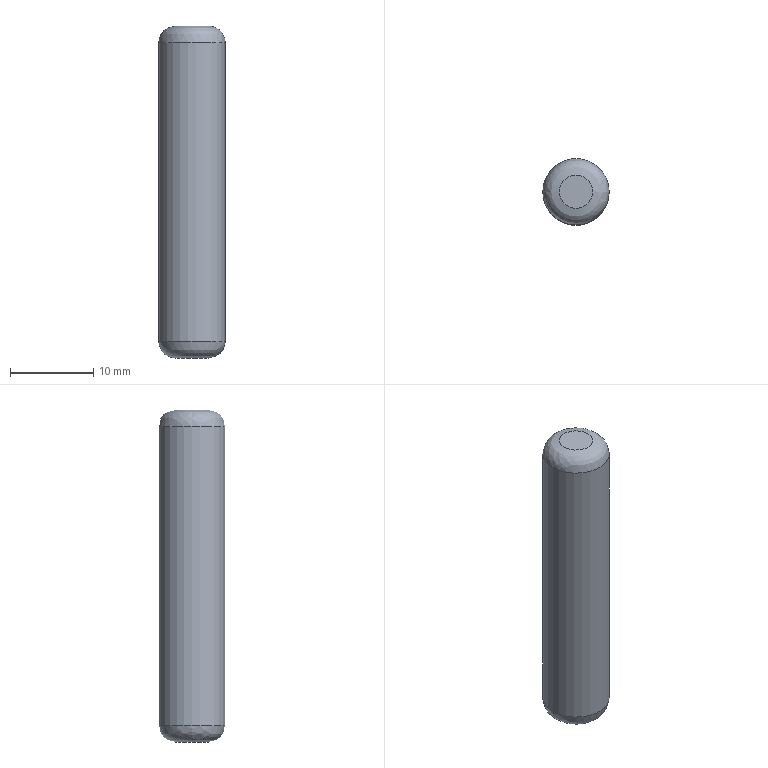Part | STEP file | Tube feed_id1738_x_t | 1 solid | 5 faces | box 8 x 8 x 40 mm | volume 1972 mm3 | plane 2 | spline 2 | cylinder 1 | commonest cylinder face diameters 8 x1
STEP:
#1=CARTESIAN_POINT('',(0.,0.,0.));
#2=DIRECTION('',(0.,0.,1.));
#3=DIRECTION('',(1.,0.,0.));
#4=AXIS2_PLACEMENT_3D('',#1,#2,#3);
#5=CARTESIAN_POINT('',(146.5,105.036,-239.5));
#6=VERTEX_POINT('',#5);
#7=CARTESIAN_POINT('',(148.5,105.036,-239.5));
#8=DIRECTION('',(0.,0.,-1.));
#9=DIRECTION('',(-1.,0.,0.));
#10=AXIS2_PLACEMENT_3D('',#7,#8,#9);
#11=CIRCLE('',#10,2.);
#12=CARTESIAN_POINT('',(148.5,105.036,-239.5));
#13=DIRECTION('',(0.,0.,-1.));
#14=DIRECTION('',(-1.,0.,0.));
#15=AXIS2_PLACEMENT_3D('',#12,#13,#14);
#16=PLANE('',#15);
#17=CARTESIAN_POINT('',(0.,0.));
#18=DIRECTION('',(1.,0.));
#19=AXIS2_PLACEMENT_2D('',#17,#18);
#20=CIRCLE('',#19,2.);
#21=(GEOMETRIC_REPRESENTATION_CONTEXT(2)PARAMETRIC_REPRESENTATION_CONTEXT()REPRESENTATION_CONTEXT('',''));
#22=DEFINITIONAL_REPRESENTATION('',(#20),#21);
#23=PCURVE('',#16,#22);
#24=CARTESIAN_POINT('',(146.5,105.036,-239.5));
#25=CARTESIAN_POINT('',(146.5,109.036,-239.5));
#26=CARTESIAN_POINT('',(150.5,109.036,-239.5));
#27=CARTESIAN_POINT('',(150.5,105.036,-239.5));
#28=CARTESIAN_POINT('',(150.5,101.036,-239.5));
#29=CARTESIAN_POINT('',(146.5,101.036,-239.5));
#30=CARTESIAN_POINT('',(146.5,105.036,-239.5));
#31=CARTESIAN_POINT('',(145.328,105.036,-239.5));
#32=CARTESIAN_POINT('',(145.328,111.379,-239.5));
#33=CARTESIAN_POINT('',(151.672,111.379,-239.5));
#34=CARTESIAN_POINT('',(151.672,105.036,-239.5));
#35=CARTESIAN_POINT('',(151.672,98.692,-239.5));
#36=CARTESIAN_POINT('',(145.328,98.692,-239.5));
#37=CARTESIAN_POINT('',(145.328,105.036,-239.5));
#38=CARTESIAN_POINT('',(144.5,105.036,-238.672));
#39=CARTESIAN_POINT('',(144.5,113.036,-238.672));
#40=CARTESIAN_POINT('',(152.5,113.036,-238.672));
#41=CARTESIAN_POINT('',(152.5,105.036,-238.672));
#42=CARTESIAN_POINT('',(152.5,97.036,-238.672));
#43=CARTESIAN_POINT('',(144.5,97.036,-238.672));
#44=CARTESIAN_POINT('',(144.5,105.036,-238.672));
#45=CARTESIAN_POINT('',(144.5,105.036,-237.5));
#46=CARTESIAN_POINT('',(144.5,113.036,-237.5));
#47=CARTESIAN_POINT('',(152.5,113.036,-237.5));
#48=CARTESIAN_POINT('',(152.5,105.036,-237.5));
#49=CARTESIAN_POINT('',(152.5,97.036,-237.5));
#50=CARTESIAN_POINT('',(144.5,97.036,-237.5));
#51=CARTESIAN_POINT('',(144.5,105.036,-237.5));
#52=(BOUNDED_SURFACE()B_SPLINE_SURFACE(3,3,((#24,#25,#26,#27,#28,#29,#30),(#31,#32,#33,#34,#35,#36,#37),(#38,#39,#40,#41,#42,#43,#44),(#45,#46,#47,#48,#49,#50,#51)),.UNSPECIFIED.,.F.,.T.,.F.)B_SPLINE_SURFACE_WITH_KNOTS((4,4),(1,3,3,3,1),(0.,1.),(-0.5,0.,0.5,1.,1.5),.UNSPECIFIED.)GEOMETRIC_REPRESENTATION_ITEM()RATIONAL_B_SPLINE_SURFACE(((1.,0.3333,0.3333,1.,0.3333,0.3333,1.),(0.8047,0.2682,0.2682,0.8047,0.2682,0.2682,0.8047),(0.8047,0.2682,0.2682,0.8047,0.2682,0.2682,0.8047),(1.,0.3333,0.3333,1.,0.3333,0.3333,1.)))REPRESENTATION_ITEM('')SURFACE());
#53=CARTESIAN_POINT('',(0.,0.));
#54=CARTESIAN_POINT('',(0.,0.02352));
#55=CARTESIAN_POINT('',(0.,0.06491));
#56=CARTESIAN_POINT('',(0.,0.1146));
#57=CARTESIAN_POINT('',(0.,0.1575));
#58=CARTESIAN_POINT('',(0.,0.196));
#59=CARTESIAN_POINT('',(0.,0.2322));
#60=CARTESIAN_POINT('',(0.,0.2678));
#61=CARTESIAN_POINT('',(0.,0.304));
#62=CARTESIAN_POINT('',(0.,0.3425));
#63=CARTESIAN_POINT('',(0.,0.3856));
#64=CARTESIAN_POINT('',(0.,0.4343));
#65=CARTESIAN_POINT('',(0.,0.5));
#66=CARTESIAN_POINT('',(0.,0.5657));
#67=CARTESIAN_POINT('',(0.,0.6144));
#68=CARTESIAN_POINT('',(0.,0.6575));
#69=CARTESIAN_POINT('',(0.,0.696));
#70=CARTESIAN_POINT('',(0.,0.7322));
#71=CARTESIAN_POINT('',(0.,0.7678));
#72=CARTESIAN_POINT('',(0.,0.804));
#73=CARTESIAN_POINT('',(0.,0.8425));
#74=CARTESIAN_POINT('',(0.,0.8854));
#75=CARTESIAN_POINT('',(0.,0.9351));
#76=CARTESIAN_POINT('',(0.,0.9765));
#77=CARTESIAN_POINT('',(0.,1.));
#78=B_SPLINE_CURVE_WITH_KNOTS('',3,(#53,#54,#55,#56,#57,#58,#59,#60,#61,#62,#63,#64,#65,#66,#67,#68,#69,#70,#71,#72,#73,#74,#75,#76,#77),.UNSPECIFIED.,.F.,.F.,(4,1,1,1,1,1,1,1,1,1,1,1,1,1,1,1,1,1,1,1,1,1,4),(0.,0.2856,0.5712,0.8568,1.142,1.428,1.714,1.999,2.285,2.57,2.856,3.142,3.427,3.713,3.998,4.284,4.57,4.855,5.141,5.426,5.712,5.998,6.283),.QUASI_UNIFORM_KNOTS.);
#79=(GEOMETRIC_REPRESENTATION_CONTEXT(2)PARAMETRIC_REPRESENTATION_CONTEXT()REPRESENTATION_CONTEXT('',''));
#80=DEFINITIONAL_REPRESENTATION('',(#78),#79);
#81=PCURVE('',#52,#80);
#82=SURFACE_CURVE('',#11,(#23,#81),.PCURVE_S1.);
#83=EDGE_CURVE('',#6,#6,#82,.T.);
#84=ORIENTED_EDGE('',*,*,#83,.T.);
#85=EDGE_LOOP('',(#84));
#86=FACE_BOUND('',#85,.T.);
#87=ADVANCED_FACE('',(#86),#16,.T.);
#88=CARTESIAN_POINT('',(150.5,105.036,-199.5));
#89=VERTEX_POINT('',#88);
#90=CARTESIAN_POINT('',(148.5,105.036,-199.5));
#91=DIRECTION('',(0.,0.,1.));
#92=DIRECTION('',(1.,0.,0.));
#93=AXIS2_PLACEMENT_3D('',#90,#91,#92);
#94=CIRCLE('',#93,2.);
#95=CARTESIAN_POINT('',(148.5,105.036,-199.5));
#96=DIRECTION('',(0.,0.,1.));
#97=DIRECTION('',(1.,0.,0.));
#98=AXIS2_PLACEMENT_3D('',#95,#96,#97);
#99=PLANE('',#98);
#100=CARTESIAN_POINT('',(0.,0.));
#101=DIRECTION('',(1.,0.));
#102=AXIS2_PLACEMENT_2D('',#100,#101);
#103=CIRCLE('',#102,2.);
#104=(GEOMETRIC_REPRESENTATION_CONTEXT(2)PARAMETRIC_REPRESENTATION_CONTEXT()REPRESENTATION_CONTEXT('',''));
#105=DEFINITIONAL_REPRESENTATION('',(#103),#104);
#106=PCURVE('',#99,#105);
#107=CARTESIAN_POINT('',(150.5,105.036,-199.5));
#108=CARTESIAN_POINT('',(150.5,109.036,-199.5));
#109=CARTESIAN_POINT('',(146.5,109.036,-199.5));
#110=CARTESIAN_POINT('',(146.5,105.036,-199.5));
#111=CARTESIAN_POINT('',(146.5,101.036,-199.5));
#112=CARTESIAN_POINT('',(150.5,101.036,-199.5));
#113=CARTESIAN_POINT('',(150.5,105.036,-199.5));
#114=CARTESIAN_POINT('',(151.672,105.036,-199.5));
#115=CARTESIAN_POINT('',(151.672,111.379,-199.5));
#116=CARTESIAN_POINT('',(145.328,111.379,-199.5));
#117=CARTESIAN_POINT('',(145.328,105.036,-199.5));
#118=CARTESIAN_POINT('',(145.328,98.692,-199.5));
#119=CARTESIAN_POINT('',(151.672,98.692,-199.5));
#120=CARTESIAN_POINT('',(151.672,105.036,-199.5));
#121=CARTESIAN_POINT('',(152.5,105.036,-200.328));
#122=CARTESIAN_POINT('',(152.5,113.036,-200.328));
#123=CARTESIAN_POINT('',(144.5,113.036,-200.328));
#124=CARTESIAN_POINT('',(144.5,105.036,-200.328));
#125=CARTESIAN_POINT('',(144.5,97.036,-200.328));
#126=CARTESIAN_POINT('',(152.5,97.036,-200.328));
#127=CARTESIAN_POINT('',(152.5,105.036,-200.328));
#128=CARTESIAN_POINT('',(152.5,105.036,-201.5));
#129=CARTESIAN_POINT('',(152.5,113.036,-201.5));
#130=CARTESIAN_POINT('',(144.5,113.036,-201.5));
#131=CARTESIAN_POINT('',(144.5,105.036,-201.5));
#132=CARTESIAN_POINT('',(144.5,97.036,-201.5));
#133=CARTESIAN_POINT('',(152.5,97.036,-201.5));
#134=CARTESIAN_POINT('',(152.5,105.036,-201.5));
#135=(BOUNDED_SURFACE()B_SPLINE_SURFACE(3,3,((#107,#108,#109,#110,#111,#112,#113),(#114,#115,#116,#117,#118,#119,#120),(#121,#122,#123,#124,#125,#126,#127),(#128,#129,#130,#131,#132,#133,#134)),.UNSPECIFIED.,.F.,.T.,.F.)B_SPLINE_SURFACE_WITH_KNOTS((4,4),(1,3,3,3,1),(0.,1.),(-0.5,0.,0.5,1.,1.5),.UNSPECIFIED.)GEOMETRIC_REPRESENTATION_ITEM()RATIONAL_B_SPLINE_SURFACE(((1.,0.3333,0.3333,1.,0.3333,0.3333,1.),(0.8047,0.2682,0.2682,0.8047,0.2682,0.2682,0.8047),(0.8047,0.2682,0.2682,0.8047,0.2682,0.2682,0.8047),(1.,0.3333,0.3333,1.,0.3333,0.3333,1.)))REPRESENTATION_ITEM('')SURFACE());
#136=CARTESIAN_POINT('',(0.,0.));
#137=CARTESIAN_POINT('',(0.,0.02352));
#138=CARTESIAN_POINT('',(0.,0.06491));
#139=CARTESIAN_POINT('',(0.,0.1146));
#140=CARTESIAN_POINT('',(0.,0.1575));
#141=CARTESIAN_POINT('',(0.,0.196));
#142=CARTESIAN_POINT('',(0.,0.2322));
#143=CARTESIAN_POINT('',(0.,0.2678));
#144=CARTESIAN_POINT('',(0.,0.304));
#145=CARTESIAN_POINT('',(0.,0.3425));
#146=CARTESIAN_POINT('',(0.,0.3856));
#147=CARTESIAN_POINT('',(0.,0.4343));
#148=CARTESIAN_POINT('',(0.,0.5));
#149=CARTESIAN_POINT('',(0.,0.5657));
#150=CARTESIAN_POINT('',(0.,0.6144));
#151=CARTESIAN_POINT('',(0.,0.6575));
#152=CARTESIAN_POINT('',(0.,0.696));
#153=CARTESIAN_POINT('',(0.,0.7322));
#154=CARTESIAN_POINT('',(0.,0.7678));
#155=CARTESIAN_POINT('',(0.,0.804));
#156=CARTESIAN_POINT('',(0.,0.8425));
#157=CARTESIAN_POINT('',(0.,0.8854));
#158=CARTESIAN_POINT('',(0.,0.9351));
#159=CARTESIAN_POINT('',(0.,0.9765));
#160=CARTESIAN_POINT('',(0.,1.));
#161=B_SPLINE_CURVE_WITH_KNOTS('',3,(#136,#137,#138,#139,#140,#141,#142,#143,#144,#145,#146,#147,#148,#149,#150,#151,#152,#153,#154,#155,#156,#157,#158,#159,#160),.UNSPECIFIED.,.F.,.F.,(4,1,1,1,1,1,1,1,1,1,1,1,1,1,1,1,1,1,1,1,1,1,4),(0.,0.2856,0.5712,0.8568,1.142,1.428,1.714,1.999,2.285,2.57,2.856,3.142,3.427,3.713,3.998,4.284,4.57,4.855,5.141,5.426,5.712,5.998,6.283),.QUASI_UNIFORM_KNOTS.);
#162=(GEOMETRIC_REPRESENTATION_CONTEXT(2)PARAMETRIC_REPRESENTATION_CONTEXT()REPRESENTATION_CONTEXT('',''));
#163=DEFINITIONAL_REPRESENTATION('',(#161),#162);
#164=PCURVE('',#135,#163);
#165=SURFACE_CURVE('',#94,(#106,#164),.PCURVE_S1.);
#166=EDGE_CURVE('',#89,#89,#165,.T.);
#167=ORIENTED_EDGE('',*,*,#166,.T.);
#168=EDGE_LOOP('',(#167));
#169=FACE_BOUND('',#168,.T.);
#170=ADVANCED_FACE('',(#169),#99,.T.);
#171=CARTESIAN_POINT('',(144.5,105.036,-237.5));
#172=VERTEX_POINT('',#171);
#173=CARTESIAN_POINT('',(152.5,105.036,-237.5));
#174=VERTEX_POINT('',#173);
#175=CARTESIAN_POINT('',(148.5,105.036,-237.5));
#176=DIRECTION('',(0.,0.,1.));
#177=DIRECTION('',(-1.,0.,0.));
#178=AXIS2_PLACEMENT_3D('',#175,#176,#177);
#179=CIRCLE('',#178,4.);
#180=CARTESIAN_POINT('',(148.5,105.036,-199.5));
#181=DIRECTION('',(0.,0.,-1.));
#182=DIRECTION('',(1.,0.,0.));
#183=AXIS2_PLACEMENT_3D('',#180,#181,#182);
#184=CYLINDRICAL_SURFACE('',#183,4.);
#185=CARTESIAN_POINT('',(3.142,38.));
#186=DIRECTION('',(-1.,0.));
#187=VECTOR('',#186,1.);
#188=LINE('',#185,#187);
#189=(GEOMETRIC_REPRESENTATION_CONTEXT(2)PARAMETRIC_REPRESENTATION_CONTEXT()REPRESENTATION_CONTEXT('',''));
#190=DEFINITIONAL_REPRESENTATION('',(#188),#189);
#191=PCURVE('',#184,#190);
#192=CARTESIAN_POINT('',(1.,1.));
#193=CARTESIAN_POINT('',(1.,0.9881));
#194=CARTESIAN_POINT('',(1.,0.966));
#195=CARTESIAN_POINT('',(1.,0.9367));
#196=CARTESIAN_POINT('',(1.,0.9103));
#197=CARTESIAN_POINT('',(1.,0.8862));
#198=CARTESIAN_POINT('',(1.,0.8639));
#199=CARTESIAN_POINT('',(1.,0.8431));
#200=CARTESIAN_POINT('',(1.,0.8233));
#201=CARTESIAN_POINT('',(1.,0.8043));
#202=CARTESIAN_POINT('',(1.,0.7859));
#203=CARTESIAN_POINT('',(1.,0.7678));
#204=CARTESIAN_POINT('',(1.,0.75));
#205=CARTESIAN_POINT('',(1.,0.7322));
#206=CARTESIAN_POINT('',(1.,0.7141));
#207=CARTESIAN_POINT('',(1.,0.6957));
#208=CARTESIAN_POINT('',(1.,0.6767));
#209=CARTESIAN_POINT('',(1.,0.6569));
#210=CARTESIAN_POINT('',(1.,0.6361));
#211=CARTESIAN_POINT('',(1.,0.6138));
#212=CARTESIAN_POINT('',(1.,0.5897));
#213=CARTESIAN_POINT('',(1.,0.5633));
#214=CARTESIAN_POINT('',(1.,0.534));
#215=CARTESIAN_POINT('',(1.,0.5119));
#216=CARTESIAN_POINT('',(1.,0.5));
#217=B_SPLINE_CURVE_WITH_KNOTS('',3,(#192,#193,#194,#195,#196,#197,#198,#199,#200,#201,#202,#203,#204,#205,#206,#207,#208,#209,#210,#211,#212,#213,#214,#215,#216),.UNSPECIFIED.,.F.,.F.,(4,1,1,1,1,1,1,1,1,1,1,1,1,1,1,1,1,1,1,1,1,1,4),(0.,0.1428,0.2856,0.4284,0.5712,0.714,0.8568,0.9996,1.142,1.285,1.428,1.571,1.714,1.856,1.999,2.142,2.285,2.428,2.57,2.713,2.856,2.999,3.142),.QUASI_UNIFORM_KNOTS.);
#218=(GEOMETRIC_REPRESENTATION_CONTEXT(2)PARAMETRIC_REPRESENTATION_CONTEXT()REPRESENTATION_CONTEXT('',''));
#219=DEFINITIONAL_REPRESENTATION('',(#217),#218);
#220=PCURVE('',#52,#219);
#221=SURFACE_CURVE('',#179,(#191,#220),.PCURVE_S1.);
#222=EDGE_CURVE('',#172,#174,#221,.T.);
#223=ORIENTED_EDGE('',*,*,#222,.T.);
#224=CARTESIAN_POINT('',(152.5,105.036,-201.5));
#225=VERTEX_POINT('',#224);
#226=CARTESIAN_POINT('',(152.5,105.036,-201.5));
#227=CARTESIAN_POINT('',(152.5,105.036,-237.5));
#228=B_SPLINE_CURVE_WITH_KNOTS('',1,(#226,#227),.UNSPECIFIED.,.F.,.F.,(2,2),(2.,38.),.PIECEWISE_BEZIER_KNOTS.);
#229=CARTESIAN_POINT('',(0.,0.));
#230=DIRECTION('',(0.,1.));
#231=VECTOR('',#230,1.);
#232=LINE('',#229,#231);
#233=(GEOMETRIC_REPRESENTATION_CONTEXT(2)PARAMETRIC_REPRESENTATION_CONTEXT()REPRESENTATION_CONTEXT('',''));
#234=DEFINITIONAL_REPRESENTATION('',(#232),#233);
#235=PCURVE('',#184,#234);
#236=CARTESIAN_POINT('',(6.283,0.));
#237=DIRECTION('',(0.,1.));
#238=VECTOR('',#237,1.);
#239=LINE('',#236,#238);
#240=(GEOMETRIC_REPRESENTATION_CONTEXT(2)PARAMETRIC_REPRESENTATION_CONTEXT()REPRESENTATION_CONTEXT('',''));
#241=DEFINITIONAL_REPRESENTATION('',(#239),#240);
#242=PCURVE('',#184,#241);
#243=SEAM_CURVE('',#228,(#235,#242),.PCURVE_S1.);
#244=EDGE_CURVE('',#225,#174,#243,.T.);
#245=ORIENTED_EDGE('',*,*,#244,.F.);
#246=CARTESIAN_POINT('',(148.5,105.036,-201.5));
#247=DIRECTION('',(0.,0.,-1.));
#248=DIRECTION('',(1.,0.,0.));
#249=AXIS2_PLACEMENT_3D('',#246,#247,#248);
#250=CIRCLE('',#249,4.);
#251=CARTESIAN_POINT('',(0.,2.));
#252=DIRECTION('',(1.,0.));
#253=VECTOR('',#252,1.);
#254=LINE('',#251,#253);
#255=(GEOMETRIC_REPRESENTATION_CONTEXT(2)PARAMETRIC_REPRESENTATION_CONTEXT()REPRESENTATION_CONTEXT('',''));
#256=DEFINITIONAL_REPRESENTATION('',(#254),#255);
#257=PCURVE('',#184,#256);
#258=CARTESIAN_POINT('',(1.,1.));
#259=CARTESIAN_POINT('',(1.,0.9765));
#260=CARTESIAN_POINT('',(1.,0.9351));
#261=CARTESIAN_POINT('',(1.,0.8854));
#262=CARTESIAN_POINT('',(1.,0.8425));
#263=CARTESIAN_POINT('',(1.,0.804));
#264=CARTESIAN_POINT('',(1.,0.7678));
#265=CARTESIAN_POINT('',(1.,0.7322));
#266=CARTESIAN_POINT('',(1.,0.696));
#267=CARTESIAN_POINT('',(1.,0.6575));
#268=CARTESIAN_POINT('',(1.,0.6144));
#269=CARTESIAN_POINT('',(1.,0.5657));
#270=CARTESIAN_POINT('',(1.,0.5));
#271=CARTESIAN_POINT('',(1.,0.4343));
#272=CARTESIAN_POINT('',(1.,0.3856));
#273=CARTESIAN_POINT('',(1.,0.3425));
#274=CARTESIAN_POINT('',(1.,0.304));
#275=CARTESIAN_POINT('',(1.,0.2678));
#276=CARTESIAN_POINT('',(1.,0.2322));
#277=CARTESIAN_POINT('',(1.,0.196));
#278=CARTESIAN_POINT('',(1.,0.1575));
#279=CARTESIAN_POINT('',(1.,0.1146));
#280=CARTESIAN_POINT('',(1.,0.06491));
#281=CARTESIAN_POINT('',(1.,0.02352));
#282=CARTESIAN_POINT('',(1.,0.));
#283=B_SPLINE_CURVE_WITH_KNOTS('',3,(#258,#259,#260,#261,#262,#263,#264,#265,#266,#267,#268,#269,#270,#271,#272,#273,#274,#275,#276,#277,#278,#279,#280,#281,#282),.UNSPECIFIED.,.F.,.F.,(4,1,1,1,1,1,1,1,1,1,1,1,1,1,1,1,1,1,1,1,1,1,4),(0.,0.2856,0.5712,0.8568,1.142,1.428,1.714,1.999,2.285,2.57,2.856,3.142,3.427,3.713,3.998,4.284,4.57,4.855,5.141,5.426,5.712,5.998,6.283),.QUASI_UNIFORM_KNOTS.);
#284=(GEOMETRIC_REPRESENTATION_CONTEXT(2)PARAMETRIC_REPRESENTATION_CONTEXT()REPRESENTATION_CONTEXT('',''));
#285=DEFINITIONAL_REPRESENTATION('',(#283),#284);
#286=PCURVE('',#135,#285);
#287=SURFACE_CURVE('',#250,(#257,#286),.PCURVE_S1.);
#288=EDGE_CURVE('',#225,#225,#287,.T.);
#289=ORIENTED_EDGE('',*,*,#288,.T.);
#290=ORIENTED_EDGE('',*,*,#244,.T.);
#291=CARTESIAN_POINT('',(148.5,105.036,-237.5));
#292=DIRECTION('',(0.,0.,1.));
#293=DIRECTION('',(-1.,0.,0.));
#294=AXIS2_PLACEMENT_3D('',#291,#292,#293);
#295=CIRCLE('',#294,4.);
#296=CARTESIAN_POINT('',(9.425,38.));
#297=DIRECTION('',(-1.,0.));
#298=VECTOR('',#297,1.);
#299=LINE('',#296,#298);
#300=(GEOMETRIC_REPRESENTATION_CONTEXT(2)PARAMETRIC_REPRESENTATION_CONTEXT()REPRESENTATION_CONTEXT('',''));
#301=DEFINITIONAL_REPRESENTATION('',(#299),#300);
#302=PCURVE('',#184,#301);
#303=CARTESIAN_POINT('',(1.,0.5));
#304=CARTESIAN_POINT('',(1.,0.4881));
#305=CARTESIAN_POINT('',(1.,0.466));
#306=CARTESIAN_POINT('',(1.,0.4367));
#307=CARTESIAN_POINT('',(1.,0.4103));
#308=CARTESIAN_POINT('',(1.,0.3862));
#309=CARTESIAN_POINT('',(1.,0.3639));
#310=CARTESIAN_POINT('',(1.,0.3431));
#311=CARTESIAN_POINT('',(1.,0.3233));
#312=CARTESIAN_POINT('',(1.,0.3043));
#313=CARTESIAN_POINT('',(1.,0.2859));
#314=CARTESIAN_POINT('',(1.,0.2678));
#315=CARTESIAN_POINT('',(1.,0.25));
#316=CARTESIAN_POINT('',(1.,0.2322));
#317=CARTESIAN_POINT('',(1.,0.2141));
#318=CARTESIAN_POINT('',(1.,0.1957));
#319=CARTESIAN_POINT('',(1.,0.1767));
#320=CARTESIAN_POINT('',(1.,0.1569));
#321=CARTESIAN_POINT('',(1.,0.1361));
#322=CARTESIAN_POINT('',(1.,0.1138));
#323=CARTESIAN_POINT('',(1.,0.08972));
#324=CARTESIAN_POINT('',(1.,0.06334));
#325=CARTESIAN_POINT('',(1.,0.03403));
#326=CARTESIAN_POINT('',(1.,0.01187));
#327=CARTESIAN_POINT('',(1.,0.));
#328=B_SPLINE_CURVE_WITH_KNOTS('',3,(#303,#304,#305,#306,#307,#308,#309,#310,#311,#312,#313,#314,#315,#316,#317,#318,#319,#320,#321,#322,#323,#324,#325,#326,#327),.UNSPECIFIED.,.F.,.F.,(4,1,1,1,1,1,1,1,1,1,1,1,1,1,1,1,1,1,1,1,1,1,4),(3.142,3.284,3.427,3.57,3.713,3.856,3.998,4.141,4.284,4.427,4.57,4.712,4.855,4.998,5.141,5.284,5.426,5.569,5.712,5.855,5.998,6.14,6.283),.QUASI_UNIFORM_KNOTS.);
#329=(GEOMETRIC_REPRESENTATION_CONTEXT(2)PARAMETRIC_REPRESENTATION_CONTEXT()REPRESENTATION_CONTEXT('',''));
#330=DEFINITIONAL_REPRESENTATION('',(#328),#329);
#331=PCURVE('',#52,#330);
#332=SURFACE_CURVE('',#295,(#302,#331),.PCURVE_S1.);
#333=EDGE_CURVE('',#174,#172,#332,.T.);
#334=ORIENTED_EDGE('',*,*,#333,.T.);
#335=EDGE_LOOP('',(#223,#245,#289,#290,#334));
#336=FACE_BOUND('',#335,.T.);
#337=ADVANCED_FACE('',(#336),#184,.T.);
#338=ORIENTED_EDGE('',*,*,#83,.F.);
#339=CARTESIAN_POINT('',(146.5,105.036,-239.5));
#340=CARTESIAN_POINT('',(145.328,105.036,-239.5));
#341=CARTESIAN_POINT('',(144.5,105.036,-238.672));
#342=CARTESIAN_POINT('',(144.5,105.036,-237.5));
#343=(BOUNDED_CURVE()B_SPLINE_CURVE(3,(#339,#340,#341,#342),.UNSPECIFIED.,.F.,.F.)B_SPLINE_CURVE_WITH_KNOTS((4,4),(0.,1.),.PIECEWISE_BEZIER_KNOTS.)CURVE()GEOMETRIC_REPRESENTATION_ITEM()RATIONAL_B_SPLINE_CURVE((1.,0.8047,0.8047,1.))REPRESENTATION_ITEM(''));
#344=CARTESIAN_POINT('',(0.,0.));
#345=DIRECTION('',(1.,0.));
#346=VECTOR('',#345,1.);
#347=LINE('',#344,#346);
#348=(GEOMETRIC_REPRESENTATION_CONTEXT(2)PARAMETRIC_REPRESENTATION_CONTEXT()REPRESENTATION_CONTEXT('',''));
#349=DEFINITIONAL_REPRESENTATION('',(#347),#348);
#350=PCURVE('',#52,#349);
#351=CARTESIAN_POINT('',(0.,1.));
#352=DIRECTION('',(1.,0.));
#353=VECTOR('',#352,1.);
#354=LINE('',#351,#353);
#355=(GEOMETRIC_REPRESENTATION_CONTEXT(2)PARAMETRIC_REPRESENTATION_CONTEXT()REPRESENTATION_CONTEXT('',''));
#356=DEFINITIONAL_REPRESENTATION('',(#354),#355);
#357=PCURVE('',#52,#356);
#358=SEAM_CURVE('',#343,(#350,#357),.PCURVE_S1.);
#359=EDGE_CURVE('',#6,#172,#358,.T.);
#360=ORIENTED_EDGE('',*,*,#359,.T.);
#361=ORIENTED_EDGE('',*,*,#333,.F.);
#362=ORIENTED_EDGE('',*,*,#222,.F.);
#363=ORIENTED_EDGE('',*,*,#359,.F.);
#364=EDGE_LOOP('',(#338,#360,#361,#362,#363));
#365=FACE_BOUND('',#364,.T.);
#366=ADVANCED_FACE('',(#365),#52,.T.);
#367=ORIENTED_EDGE('',*,*,#166,.F.);
#368=CARTESIAN_POINT('',(150.5,105.036,-199.5));
#369=CARTESIAN_POINT('',(151.672,105.036,-199.5));
#370=CARTESIAN_POINT('',(152.5,105.036,-200.328));
#371=CARTESIAN_POINT('',(152.5,105.036,-201.5));
#372=(BOUNDED_CURVE()B_SPLINE_CURVE(3,(#368,#369,#370,#371),.UNSPECIFIED.,.F.,.F.)B_SPLINE_CURVE_WITH_KNOTS((4,4),(0.,1.),.PIECEWISE_BEZIER_KNOTS.)CURVE()GEOMETRIC_REPRESENTATION_ITEM()RATIONAL_B_SPLINE_CURVE((1.,0.8047,0.8047,1.))REPRESENTATION_ITEM(''));
#373=CARTESIAN_POINT('',(0.,0.));
#374=DIRECTION('',(1.,0.));
#375=VECTOR('',#374,1.);
#376=LINE('',#373,#375);
#377=(GEOMETRIC_REPRESENTATION_CONTEXT(2)PARAMETRIC_REPRESENTATION_CONTEXT()REPRESENTATION_CONTEXT('',''));
#378=DEFINITIONAL_REPRESENTATION('',(#376),#377);
#379=PCURVE('',#135,#378);
#380=CARTESIAN_POINT('',(0.,1.));
#381=DIRECTION('',(1.,0.));
#382=VECTOR('',#381,1.);
#383=LINE('',#380,#382);
#384=(GEOMETRIC_REPRESENTATION_CONTEXT(2)PARAMETRIC_REPRESENTATION_CONTEXT()REPRESENTATION_CONTEXT('',''));
#385=DEFINITIONAL_REPRESENTATION('',(#383),#384);
#386=PCURVE('',#135,#385);
#387=SEAM_CURVE('',#372,(#379,#386),.PCURVE_S1.);
#388=EDGE_CURVE('',#89,#225,#387,.T.);
#389=ORIENTED_EDGE('',*,*,#388,.T.);
#390=ORIENTED_EDGE('',*,*,#288,.F.);
#391=ORIENTED_EDGE('',*,*,#388,.F.);
#392=EDGE_LOOP('',(#367,#389,#390,#391));
#393=FACE_BOUND('',#392,.T.);
#394=ADVANCED_FACE('',(#393),#135,.T.);
#395=CLOSED_SHELL('',(#87,#170,#337,#366,#394));
#396=MANIFOLD_SOLID_BREP('',#395);
#397=(LENGTH_UNIT()NAMED_UNIT(*)SI_UNIT(.MILLI.,.METRE.));
#398=UNCERTAINTY_MEASURE_WITH_UNIT(LENGTH_MEASURE(0.00001),#397,'','');
#399=(NAMED_UNIT(*)PLANE_ANGLE_UNIT()SI_UNIT($,.RADIAN.));
#400=(NAMED_UNIT(*)SI_UNIT($,.STERADIAN.)SOLID_ANGLE_UNIT());
#401=(GEOMETRIC_REPRESENTATION_CONTEXT(3)GLOBAL_UNCERTAINTY_ASSIGNED_CONTEXT((#398))GLOBAL_UNIT_ASSIGNED_CONTEXT((#397,#399,#400))REPRESENTATION_CONTEXT('',''));
#402=ADVANCED_BREP_SHAPE_REPRESENTATION('',(#4,#396),#401);